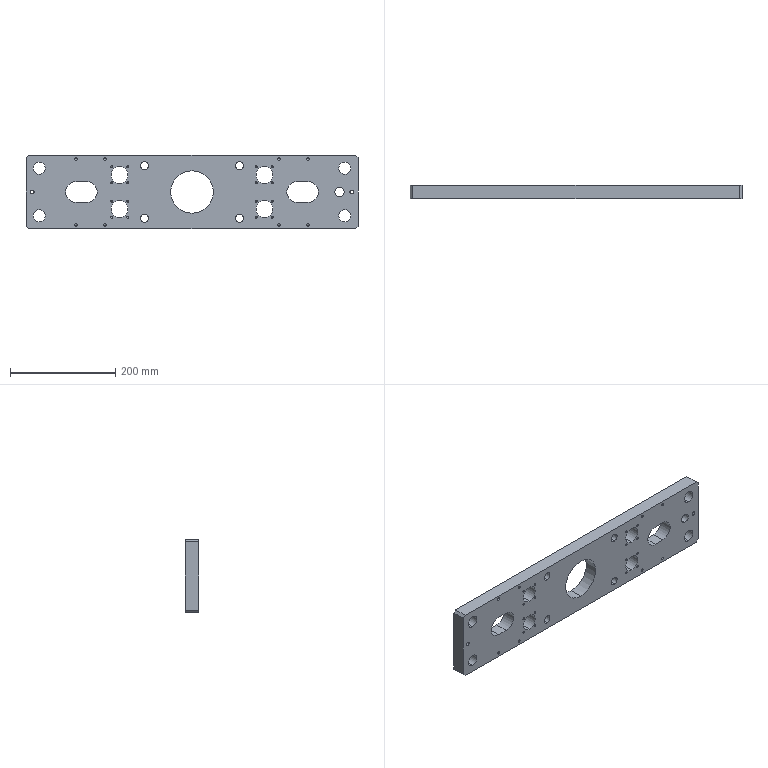Part | SolidWorks | features BaseBody 1 | 1 solid | 230 faces | box 630 x 25 x 140 mm | volume 1806087 mm3 | cylinder 128 | cone 84 | plane 18 | commonest cylinder face diameters 4.2 x32 5 x24 2.5 x8 3.3 x8 6 x8 6.8 x8